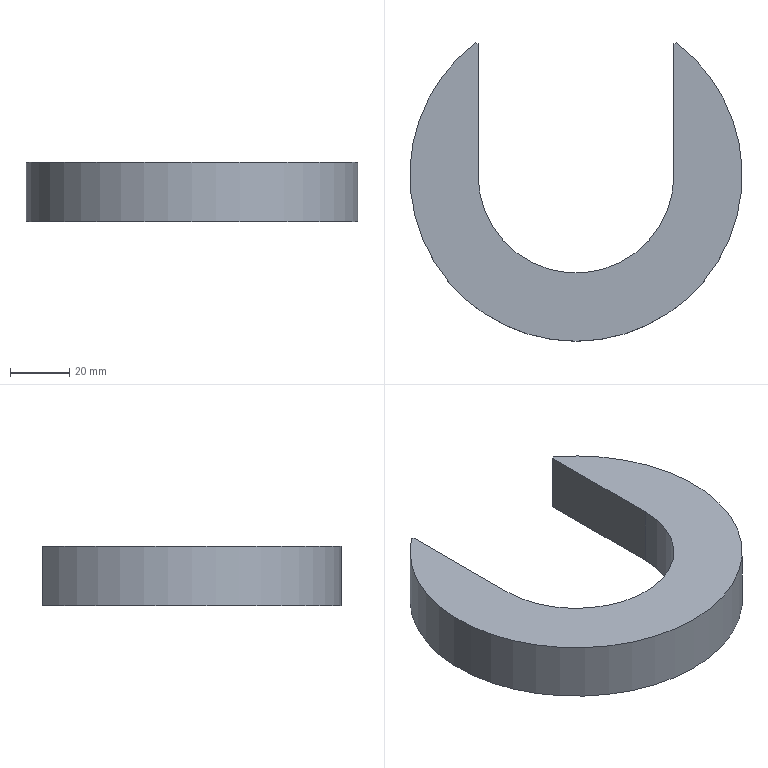Part | NX | features solid 2 | 1 solid | 8 faces | box 112 x 100.638 x 20 mm | volume 93427 mm3 | plane 6 | cylinder 2 | commonest cylinder face diameters 66 x1 112 x1
STEP:
#1=CARTESIAN_POINT('',(643.,260.,0.));
#2=VERTEX_POINT('',#1);
#3=CARTESIAN_POINT('',(577.,260.,0.));
#4=VERTEX_POINT('',#3);
#5=CARTESIAN_POINT('',(610.,260.,0.));
#6=DIRECTION('',(0.,0.,-1.));
#7=DIRECTION('',(1.,0.,0.));
#8=AXIS2_PLACEMENT_3D('',#5,#6,#7);
#9=CIRCLE('',#8,33.);
#10=EDGE_CURVE('',#2,#4,#9,.T.);
#11=ORIENTED_EDGE('',*,*,#10,.F.);
#12=CARTESIAN_POINT('',(643.,260.,-20.));
#13=VERTEX_POINT('',#12);
#14=CARTESIAN_POINT('',(643.,260.,-100.));
#15=DIRECTION('',(0.,0.,1.));
#16=VECTOR('',#15,1000.);
#17=LINE('',#14,#16);
#18=EDGE_CURVE('',#13,#2,#17,.T.);
#19=ORIENTED_EDGE('',*,*,#18,.F.);
#20=CARTESIAN_POINT('',(577.,260.,-20.));
#21=VERTEX_POINT('',#20);
#22=CARTESIAN_POINT('',(610.,260.,-20.));
#23=DIRECTION('',(0.,0.,-1.));
#24=DIRECTION('',(1.,0.,0.));
#25=AXIS2_PLACEMENT_3D('',#22,#23,#24);
#26=CIRCLE('',#25,33.);
#27=EDGE_CURVE('',#13,#21,#26,.T.);
#28=ORIENTED_EDGE('',*,*,#27,.T.);
#29=CARTESIAN_POINT('',(577.,260.,-100.));
#30=DIRECTION('',(0.,0.,1.));
#31=VECTOR('',#30,1000.);
#32=LINE('',#29,#31);
#33=EDGE_CURVE('',#21,#4,#32,.T.);
#34=ORIENTED_EDGE('',*,*,#33,.T.);
#35=EDGE_LOOP('',(#11,#19,#28,#34));
#36=FACE_BOUND('',#35,.T.);
#37=CARTESIAN_POINT('',(610.,260.,-20.));
#38=DIRECTION('',(0.,0.,1.));
#39=DIRECTION('',(1.,0.,0.));
#40=AXIS2_PLACEMENT_3D('',#37,#38,#39);
#41=CYLINDRICAL_SURFACE('',#40,33.);
#42=ADVANCED_FACE('',(#36),#41,.F.);
#43=CARTESIAN_POINT('',(643.815,304.638,-20.));
#44=VERTEX_POINT('',#43);
#45=CARTESIAN_POINT('',(576.185,304.638,-20.));
#46=VERTEX_POINT('',#45);
#47=CARTESIAN_POINT('',(610.,260.,-20.));
#48=DIRECTION('',(0.,0.,-1.));
#49=DIRECTION('',(1.,0.,0.));
#50=AXIS2_PLACEMENT_3D('',#47,#48,#49);
#51=CIRCLE('',#50,56.);
#52=EDGE_CURVE('',#44,#46,#51,.T.);
#53=ORIENTED_EDGE('',*,*,#52,.F.);
#54=CARTESIAN_POINT('',(643.815,304.638,0.));
#55=VERTEX_POINT('',#54);
#56=CARTESIAN_POINT('',(643.815,304.638,-20.));
#57=DIRECTION('',(0.,0.,1.));
#58=VECTOR('',#57,1000.);
#59=LINE('',#56,#58);
#60=EDGE_CURVE('',#55,#44,#59,.F.);
#61=ORIENTED_EDGE('',*,*,#60,.F.);
#62=CARTESIAN_POINT('',(576.185,304.638,0.));
#63=VERTEX_POINT('',#62);
#64=CARTESIAN_POINT('',(610.,260.,0.));
#65=DIRECTION('',(0.,0.,-1.));
#66=DIRECTION('',(1.,0.,0.));
#67=AXIS2_PLACEMENT_3D('',#64,#65,#66);
#68=CIRCLE('',#67,56.);
#69=EDGE_CURVE('',#55,#63,#68,.T.);
#70=ORIENTED_EDGE('',*,*,#69,.T.);
#71=CARTESIAN_POINT('',(576.185,304.638,-20.));
#72=DIRECTION('',(0.,0.,1.));
#73=VECTOR('',#72,1000.);
#74=LINE('',#71,#73);
#75=EDGE_CURVE('',#46,#63,#74,.T.);
#76=ORIENTED_EDGE('',*,*,#75,.F.);
#77=EDGE_LOOP('',(#53,#61,#70,#76));
#78=FACE_BOUND('',#77,.T.);
#79=CARTESIAN_POINT('',(610.,260.,-20.));
#80=DIRECTION('',(0.,0.,1.));
#81=DIRECTION('',(1.,0.,0.));
#82=AXIS2_PLACEMENT_3D('',#79,#80,#81);
#83=CYLINDRICAL_SURFACE('',#82,56.);
#84=ADVANCED_FACE('',(#78),#83,.T.);
#85=CARTESIAN_POINT('',(577.,304.232,-20.));
#86=VERTEX_POINT('',#85);
#87=CARTESIAN_POINT('',(577.,260.,-20.));
#88=DIRECTION('',(0.,1.,0.));
#89=VECTOR('',#88,1000.);
#90=LINE('',#87,#89);
#91=EDGE_CURVE('',#21,#86,#90,.T.);
#92=ORIENTED_EDGE('',*,*,#91,.F.);
#93=ORIENTED_EDGE('',*,*,#27,.F.);
#94=CARTESIAN_POINT('',(643.,304.232,-20.));
#95=VERTEX_POINT('',#94);
#96=CARTESIAN_POINT('',(643.,260.,-20.));
#97=DIRECTION('',(0.,1.,0.));
#98=VECTOR('',#97,1000.);
#99=LINE('',#96,#98);
#100=EDGE_CURVE('',#13,#95,#99,.T.);
#101=ORIENTED_EDGE('',*,*,#100,.T.);
#102=CARTESIAN_POINT('',(643.815,304.638,-20.));
#103=DIRECTION('',(-0.8955,-0.4451,0.));
#104=VECTOR('',#103,1000.);
#105=LINE('',#102,#104);
#106=EDGE_CURVE('',#44,#95,#105,.T.);
#107=ORIENTED_EDGE('',*,*,#106,.F.);
#108=ORIENTED_EDGE('',*,*,#52,.T.);
#109=CARTESIAN_POINT('',(577.,304.232,-20.));
#110=DIRECTION('',(-0.8955,0.4451,0.));
#111=VECTOR('',#110,1000.);
#112=LINE('',#109,#111);
#113=EDGE_CURVE('',#86,#46,#112,.T.);
#114=ORIENTED_EDGE('',*,*,#113,.F.);
#115=EDGE_LOOP('',(#92,#93,#101,#107,#108,#114));
#116=FACE_BOUND('',#115,.T.);
#117=CARTESIAN_POINT('',(610.,260.,-20.));
#118=DIRECTION('',(0.,0.,1.));
#119=DIRECTION('',(1.,0.,0.));
#120=AXIS2_PLACEMENT_3D('',#117,#118,#119);
#121=PLANE('',#120);
#122=ADVANCED_FACE('',(#116),#121,.F.);
#123=ORIENTED_EDGE('',*,*,#69,.F.);
#124=CARTESIAN_POINT('',(643.,304.232,0.));
#125=VERTEX_POINT('',#124);
#126=CARTESIAN_POINT('',(598.908,282.319,0.));
#127=DIRECTION('',(0.8955,0.4451,0.));
#128=VECTOR('',#127,1000.);
#129=LINE('',#126,#128);
#130=EDGE_CURVE('',#125,#55,#129,.T.);
#131=ORIENTED_EDGE('',*,*,#130,.F.);
#132=CARTESIAN_POINT('',(643.,260.,0.));
#133=DIRECTION('',(0.,1.,0.));
#134=VECTOR('',#133,1000.);
#135=LINE('',#132,#134);
#136=EDGE_CURVE('',#2,#125,#135,.T.);
#137=ORIENTED_EDGE('',*,*,#136,.F.);
#138=ORIENTED_EDGE('',*,*,#10,.T.);
#139=CARTESIAN_POINT('',(577.,304.232,0.));
#140=VERTEX_POINT('',#139);
#141=CARTESIAN_POINT('',(577.,260.,0.));
#142=DIRECTION('',(0.,-1.,0.));
#143=VECTOR('',#142,1000.);
#144=LINE('',#141,#143);
#145=EDGE_CURVE('',#4,#140,#144,.F.);
#146=ORIENTED_EDGE('',*,*,#145,.T.);
#147=CARTESIAN_POINT('',(621.092,282.319,0.));
#148=DIRECTION('',(0.8955,-0.4451,0.));
#149=VECTOR('',#148,1000.);
#150=LINE('',#147,#149);
#151=EDGE_CURVE('',#63,#140,#150,.T.);
#152=ORIENTED_EDGE('',*,*,#151,.F.);
#153=EDGE_LOOP('',(#123,#131,#137,#138,#146,#152));
#154=FACE_BOUND('',#153,.T.);
#155=CARTESIAN_POINT('',(610.,260.,0.));
#156=DIRECTION('',(0.,0.,1.));
#157=DIRECTION('',(1.,0.,0.));
#158=AXIS2_PLACEMENT_3D('',#155,#156,#157);
#159=PLANE('',#158);
#160=ADVANCED_FACE('',(#154),#159,.T.);
#161=ORIENTED_EDGE('',*,*,#100,.F.);
#162=ORIENTED_EDGE('',*,*,#18,.T.);
#163=ORIENTED_EDGE('',*,*,#136,.T.);
#164=CARTESIAN_POINT('',(643.,304.232,-100.));
#165=DIRECTION('',(0.,0.,1.));
#166=VECTOR('',#165,1000.);
#167=LINE('',#164,#166);
#168=EDGE_CURVE('',#95,#125,#167,.T.);
#169=ORIENTED_EDGE('',*,*,#168,.F.);
#170=EDGE_LOOP('',(#161,#162,#163,#169));
#171=FACE_BOUND('',#170,.T.);
#172=CARTESIAN_POINT('',(643.,260.,-100.));
#173=DIRECTION('',(-1.,0.,0.));
#174=DIRECTION('',(0.,0.,1.));
#175=AXIS2_PLACEMENT_3D('',#172,#173,#174);
#176=PLANE('',#175);
#177=ADVANCED_FACE('',(#171),#176,.T.);
#178=ORIENTED_EDGE('',*,*,#145,.F.);
#179=ORIENTED_EDGE('',*,*,#33,.F.);
#180=ORIENTED_EDGE('',*,*,#91,.T.);
#181=CARTESIAN_POINT('',(577.,304.232,-20.));
#182=DIRECTION('',(0.,0.,-1.));
#183=VECTOR('',#182,1000.);
#184=LINE('',#181,#183);
#185=EDGE_CURVE('',#140,#86,#184,.T.);
#186=ORIENTED_EDGE('',*,*,#185,.F.);
#187=EDGE_LOOP('',(#178,#179,#180,#186));
#188=FACE_BOUND('',#187,.T.);
#189=CARTESIAN_POINT('',(577.,260.,-100.));
#190=DIRECTION('',(-1.,0.,0.));
#191=DIRECTION('',(0.,0.,1.));
#192=AXIS2_PLACEMENT_3D('',#189,#190,#191);
#193=PLANE('',#192);
#194=ADVANCED_FACE('',(#188),#193,.F.);
#195=ORIENTED_EDGE('',*,*,#151,.T.);
#196=ORIENTED_EDGE('',*,*,#185,.T.);
#197=ORIENTED_EDGE('',*,*,#113,.T.);
#198=ORIENTED_EDGE('',*,*,#75,.T.);
#199=EDGE_LOOP('',(#195,#196,#197,#198));
#200=FACE_BOUND('',#199,.T.);
#201=CARTESIAN_POINT('',(577.,304.232,-20.));
#202=DIRECTION('',(0.4451,0.8955,0.));
#203=DIRECTION('',(0.8955,-0.4451,0.));
#204=AXIS2_PLACEMENT_3D('',#201,#202,#203);
#205=PLANE('',#204);
#206=ADVANCED_FACE('',(#200),#205,.T.);
#207=ORIENTED_EDGE('',*,*,#130,.T.);
#208=ORIENTED_EDGE('',*,*,#60,.T.);
#209=ORIENTED_EDGE('',*,*,#106,.T.);
#210=ORIENTED_EDGE('',*,*,#168,.T.);
#211=EDGE_LOOP('',(#207,#208,#209,#210));
#212=FACE_BOUND('',#211,.T.);
#213=CARTESIAN_POINT('',(643.815,304.638,-20.));
#214=DIRECTION('',(-0.4451,0.8955,0.));
#215=DIRECTION('',(0.8955,0.4451,0.));
#216=AXIS2_PLACEMENT_3D('',#213,#214,#215);
#217=PLANE('',#216);
#218=ADVANCED_FACE('',(#212),#217,.T.);
#219=CLOSED_SHELL('',(#42,#84,#122,#160,#177,#194,#206,#218));
#220=MANIFOLD_SOLID_BREP('',#219);
#221=(LENGTH_UNIT()NAMED_UNIT(*)SI_UNIT(.MILLI.,.METRE.));
#222=UNCERTAINTY_MEASURE_WITH_UNIT(LENGTH_MEASURE(0.00001),#221,'','');
#223=(NAMED_UNIT(*)PLANE_ANGLE_UNIT()SI_UNIT($,.RADIAN.));
#224=(NAMED_UNIT(*)SI_UNIT($,.STERADIAN.)SOLID_ANGLE_UNIT());
#225=(GEOMETRIC_REPRESENTATION_CONTEXT(3)GLOBAL_UNCERTAINTY_ASSIGNED_CONTEXT((#222))GLOBAL_UNIT_ASSIGNED_CONTEXT((#221,#223,#224))REPRESENTATION_CONTEXT('',''));
#226=ADVANCED_BREP_SHAPE_REPRESENTATION('',(#220),#225);